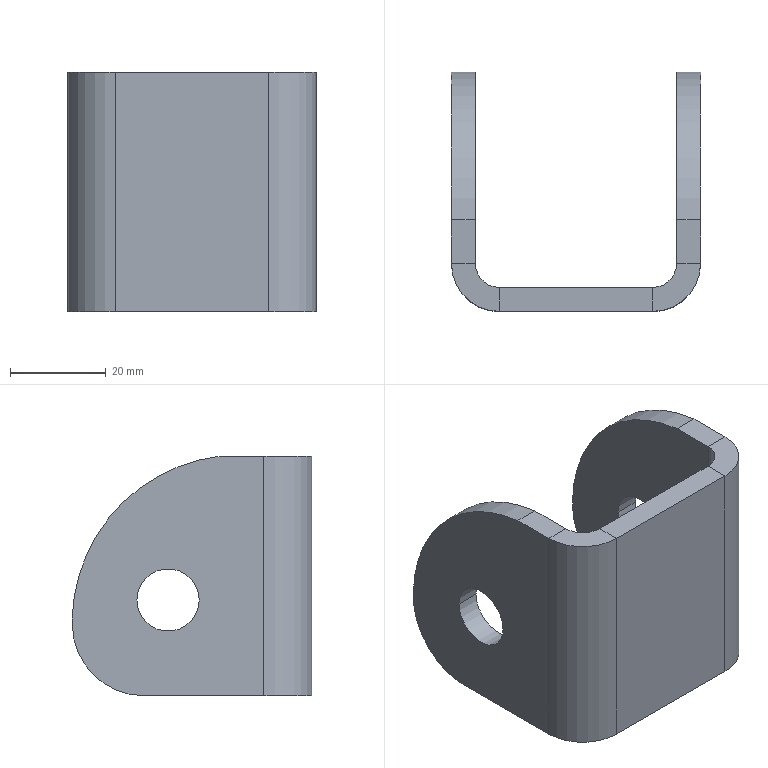Part | SolidWorks | features ICE 2, EdgeFlange 1, FlatPattern 1, SMBaseFlange 1, SheetMetal 1 | 1 solid | 30 faces | box 52 x 50 x 50 mm | volume 29535 mm3 | plane 18 | cylinder 12 | commonest cylinder face diameters 13 x4 10 x2 20 x2 30 x2 70 x2
STEP:
#1=CARTESIAN_POINT('',(26.,31.5,-5.));
#2=VERTEX_POINT('',#1);
#3=CARTESIAN_POINT('',(26.,18.5,-5.));
#4=VERTEX_POINT('',#3);
#5=CARTESIAN_POINT('',(26.,25.,-5.));
#6=DIRECTION('',(-1.,0.,0.));
#7=DIRECTION('',(0.,-1.,0.));
#8=AXIS2_PLACEMENT_3D('',#5,#6,#7);
#9=CIRCLE('',#8,6.5);
#10=EDGE_CURVE('',#2,#4,#9,.T.);
#11=ORIENTED_EDGE('',*,*,#10,.F.);
#12=CARTESIAN_POINT('',(21.,31.5,-5.));
#13=VERTEX_POINT('',#12);
#14=CARTESIAN_POINT('',(26.,31.5,-5.));
#15=DIRECTION('',(-1.,0.,0.));
#16=VECTOR('',#15,1000.);
#17=LINE('',#14,#16);
#18=EDGE_CURVE('',#2,#13,#17,.T.);
#19=ORIENTED_EDGE('',*,*,#18,.T.);
#20=CARTESIAN_POINT('',(21.,18.5,-5.));
#21=VERTEX_POINT('',#20);
#22=CARTESIAN_POINT('',(21.,25.,-5.));
#23=DIRECTION('',(1.,0.,0.));
#24=DIRECTION('',(0.,1.,0.));
#25=AXIS2_PLACEMENT_3D('',#22,#23,#24);
#26=CIRCLE('',#25,6.5);
#27=EDGE_CURVE('',#21,#13,#26,.T.);
#28=ORIENTED_EDGE('',*,*,#27,.F.);
#29=CARTESIAN_POINT('',(26.,18.5,-5.));
#30=DIRECTION('',(-1.,0.,0.));
#31=VECTOR('',#30,1000.);
#32=LINE('',#29,#31);
#33=EDGE_CURVE('',#4,#21,#32,.T.);
#34=ORIENTED_EDGE('',*,*,#33,.F.);
#35=EDGE_LOOP('',(#11,#19,#28,#34));
#36=FACE_OUTER_BOUND('',#35,.T.);
#37=CARTESIAN_POINT('',(26.,25.,-5.));
#38=DIRECTION('',(-1.,0.,0.));
#39=DIRECTION('',(0.,-1.,0.));
#40=AXIS2_PLACEMENT_3D('',#37,#38,#39);
#41=CYLINDRICAL_SURFACE('',#40,6.5);
#42=ADVANCED_FACE('',(#36),#41,.F.);
#43=CARTESIAN_POINT('',(-21.,18.5,-5.));
#44=VERTEX_POINT('',#43);
#45=CARTESIAN_POINT('',(-21.,31.5,-5.));
#46=VERTEX_POINT('',#45);
#47=CARTESIAN_POINT('',(-21.,25.,-5.));
#48=DIRECTION('',(1.,0.,0.));
#49=DIRECTION('',(0.,1.,0.));
#50=AXIS2_PLACEMENT_3D('',#47,#48,#49);
#51=CIRCLE('',#50,6.5);
#52=EDGE_CURVE('',#44,#46,#51,.T.);
#53=ORIENTED_EDGE('',*,*,#52,.T.);
#54=CARTESIAN_POINT('',(-26.,31.5,-5.));
#55=VERTEX_POINT('',#54);
#56=CARTESIAN_POINT('',(26.,31.5,-5.));
#57=DIRECTION('',(-1.,0.,0.));
#58=VECTOR('',#57,1000.);
#59=LINE('',#56,#58);
#60=EDGE_CURVE('',#46,#55,#59,.T.);
#61=ORIENTED_EDGE('',*,*,#60,.T.);
#62=CARTESIAN_POINT('',(-26.,18.5,-5.));
#63=VERTEX_POINT('',#62);
#64=CARTESIAN_POINT('',(-26.,25.,-5.));
#65=DIRECTION('',(-1.,0.,0.));
#66=DIRECTION('',(0.,-1.,0.));
#67=AXIS2_PLACEMENT_3D('',#64,#65,#66);
#68=CIRCLE('',#67,6.5);
#69=EDGE_CURVE('',#55,#63,#68,.T.);
#70=ORIENTED_EDGE('',*,*,#69,.T.);
#71=CARTESIAN_POINT('',(26.,18.5,-5.));
#72=DIRECTION('',(-1.,0.,0.));
#73=VECTOR('',#72,1000.);
#74=LINE('',#71,#73);
#75=EDGE_CURVE('',#44,#63,#74,.T.);
#76=ORIENTED_EDGE('',*,*,#75,.F.);
#77=EDGE_LOOP('',(#53,#61,#70,#76));
#78=FACE_OUTER_BOUND('',#77,.T.);
#79=CARTESIAN_POINT('',(26.,25.,-5.));
#80=DIRECTION('',(-1.,0.,0.));
#81=DIRECTION('',(0.,-1.,0.));
#82=AXIS2_PLACEMENT_3D('',#79,#80,#81);
#83=CYLINDRICAL_SURFACE('',#82,6.5);
#84=ADVANCED_FACE('',(#78),#83,.F.);
#85=CARTESIAN_POINT('',(21.,30.,-25.));
#86=VERTEX_POINT('',#85);
#87=CARTESIAN_POINT('',(21.,5.,-25.));
#88=VERTEX_POINT('',#87);
#89=CARTESIAN_POINT('',(21.,0.,-25.));
#90=DIRECTION('',(0.,-1.,0.));
#91=VECTOR('',#90,1000.);
#92=LINE('',#89,#91);
#93=EDGE_CURVE('',#86,#88,#92,.T.);
#94=ORIENTED_EDGE('',*,*,#93,.F.);
#95=CARTESIAN_POINT('',(26.,30.,-25.));
#96=VERTEX_POINT('',#95);
#97=CARTESIAN_POINT('',(26.,30.,-25.));
#98=DIRECTION('',(-1.,0.,0.));
#99=VECTOR('',#98,1000.);
#100=LINE('',#97,#99);
#101=EDGE_CURVE('',#96,#86,#100,.T.);
#102=ORIENTED_EDGE('',*,*,#101,.F.);
#103=CARTESIAN_POINT('',(26.,5.,-25.));
#104=VERTEX_POINT('',#103);
#105=CARTESIAN_POINT('',(26.,0.,-25.));
#106=DIRECTION('',(0.,-1.,0.));
#107=VECTOR('',#106,1000.);
#108=LINE('',#105,#107);
#109=EDGE_CURVE('',#96,#104,#108,.T.);
#110=ORIENTED_EDGE('',*,*,#109,.T.);
#111=CARTESIAN_POINT('',(21.,5.,-25.));
#112=DIRECTION('',(1.,0.,0.));
#113=VECTOR('',#112,1000.);
#114=LINE('',#111,#113);
#115=EDGE_CURVE('',#88,#104,#114,.T.);
#116=ORIENTED_EDGE('',*,*,#115,.F.);
#117=EDGE_LOOP('',(#94,#102,#110,#116));
#118=FACE_OUTER_BOUND('',#117,.T.);
#119=CARTESIAN_POINT('',(26.,0.,-25.));
#120=DIRECTION('',(0.,0.,-1.));
#121=DIRECTION('',(0.,1.,0.));
#122=AXIS2_PLACEMENT_3D('',#119,#120,#121);
#123=PLANE('',#122);
#124=ADVANCED_FACE('',(#118),#123,.T.);
#125=CARTESIAN_POINT('',(-26.,5.,-25.));
#126=VERTEX_POINT('',#125);
#127=CARTESIAN_POINT('',(-26.,30.,-25.));
#128=VERTEX_POINT('',#127);
#129=CARTESIAN_POINT('',(-26.,0.,-25.));
#130=DIRECTION('',(0.,1.,0.));
#131=VECTOR('',#130,1000.);
#132=LINE('',#129,#131);
#133=EDGE_CURVE('',#126,#128,#132,.T.);
#134=ORIENTED_EDGE('',*,*,#133,.T.);
#135=CARTESIAN_POINT('',(-21.,30.,-25.));
#136=VERTEX_POINT('',#135);
#137=CARTESIAN_POINT('',(26.,30.,-25.));
#138=DIRECTION('',(-1.,0.,0.));
#139=VECTOR('',#138,1000.);
#140=LINE('',#137,#139);
#141=EDGE_CURVE('',#136,#128,#140,.T.);
#142=ORIENTED_EDGE('',*,*,#141,.F.);
#143=CARTESIAN_POINT('',(-21.,5.,-25.));
#144=VERTEX_POINT('',#143);
#145=CARTESIAN_POINT('',(-21.,0.,-25.));
#146=DIRECTION('',(0.,1.,0.));
#147=VECTOR('',#146,1000.);
#148=LINE('',#145,#147);
#149=EDGE_CURVE('',#144,#136,#148,.T.);
#150=ORIENTED_EDGE('',*,*,#149,.F.);
#151=CARTESIAN_POINT('',(-26.,5.,-25.));
#152=DIRECTION('',(-1.,0.,0.));
#153=VECTOR('',#152,1000.);
#154=LINE('',#151,#153);
#155=EDGE_CURVE('',#144,#126,#154,.T.);
#156=ORIENTED_EDGE('',*,*,#155,.T.);
#157=EDGE_LOOP('',(#134,#142,#150,#156));
#158=FACE_OUTER_BOUND('',#157,.T.);
#159=CARTESIAN_POINT('',(-26.,0.,-25.));
#160=DIRECTION('',(0.,0.,-1.));
#161=DIRECTION('',(-1.,0.,0.));
#162=AXIS2_PLACEMENT_3D('',#159,#160,#161);
#163=PLANE('',#162);
#164=ADVANCED_FACE('',(#158),#163,.T.);
#165=CARTESIAN_POINT('',(-16.,-5.,25.));
#166=VERTEX_POINT('',#165);
#167=CARTESIAN_POINT('',(-16.,-5.,-25.));
#168=VERTEX_POINT('',#167);
#169=CARTESIAN_POINT('',(-16.,-5.,25.));
#170=DIRECTION('',(0.,0.,-1.));
#171=VECTOR('',#170,1000.);
#172=LINE('',#169,#171);
#173=EDGE_CURVE('',#166,#168,#172,.T.);
#174=ORIENTED_EDGE('',*,*,#173,.T.);
#175=CARTESIAN_POINT('',(16.,-5.,-25.));
#176=VERTEX_POINT('',#175);
#177=CARTESIAN_POINT('',(-26.,-5.,-25.));
#178=DIRECTION('',(-1.,0.,0.));
#179=VECTOR('',#178,1000.);
#180=LINE('',#177,#179);
#181=EDGE_CURVE('',#176,#168,#180,.T.);
#182=ORIENTED_EDGE('',*,*,#181,.F.);
#183=CARTESIAN_POINT('',(16.,-5.,25.));
#184=VERTEX_POINT('',#183);
#185=CARTESIAN_POINT('',(16.,-5.,-25.));
#186=DIRECTION('',(0.,0.,1.));
#187=VECTOR('',#186,1000.);
#188=LINE('',#185,#187);
#189=EDGE_CURVE('',#176,#184,#188,.T.);
#190=ORIENTED_EDGE('',*,*,#189,.T.);
#191=CARTESIAN_POINT('',(-26.,-5.,25.));
#192=DIRECTION('',(1.,0.,0.));
#193=VECTOR('',#192,1000.);
#194=LINE('',#191,#193);
#195=EDGE_CURVE('',#166,#184,#194,.T.);
#196=ORIENTED_EDGE('',*,*,#195,.F.);
#197=EDGE_LOOP('',(#174,#182,#190,#196));
#198=FACE_OUTER_BOUND('',#197,.T.);
#199=CARTESIAN_POINT('',(0.,-5.,0.));
#200=DIRECTION('',(0.,1.,0.));
#201=DIRECTION('',(0.,0.,1.));
#202=AXIS2_PLACEMENT_3D('',#199,#200,#201);
#203=PLANE('',#202);
#204=ADVANCED_FACE('',(#198),#203,.F.);
#205=CARTESIAN_POINT('',(16.,0.,-25.));
#206=VERTEX_POINT('',#205);
#207=CARTESIAN_POINT('',(-16.,0.,-25.));
#208=VERTEX_POINT('',#207);
#209=CARTESIAN_POINT('',(-26.,0.,-25.));
#210=DIRECTION('',(-1.,0.,0.));
#211=VECTOR('',#210,1000.);
#212=LINE('',#209,#211);
#213=EDGE_CURVE('',#206,#208,#212,.T.);
#214=ORIENTED_EDGE('',*,*,#213,.T.);
#215=CARTESIAN_POINT('',(-16.,0.,25.));
#216=VERTEX_POINT('',#215);
#217=CARTESIAN_POINT('',(-16.,0.,25.));
#218=DIRECTION('',(0.,0.,-1.));
#219=VECTOR('',#218,1000.);
#220=LINE('',#217,#219);
#221=EDGE_CURVE('',#216,#208,#220,.T.);
#222=ORIENTED_EDGE('',*,*,#221,.F.);
#223=CARTESIAN_POINT('',(16.,0.,25.));
#224=VERTEX_POINT('',#223);
#225=CARTESIAN_POINT('',(-26.,0.,25.));
#226=DIRECTION('',(1.,0.,0.));
#227=VECTOR('',#226,1000.);
#228=LINE('',#225,#227);
#229=EDGE_CURVE('',#216,#224,#228,.T.);
#230=ORIENTED_EDGE('',*,*,#229,.T.);
#231=CARTESIAN_POINT('',(16.,0.,-25.));
#232=DIRECTION('',(0.,0.,1.));
#233=VECTOR('',#232,1000.);
#234=LINE('',#231,#233);
#235=EDGE_CURVE('',#206,#224,#234,.T.);
#236=ORIENTED_EDGE('',*,*,#235,.F.);
#237=EDGE_LOOP('',(#214,#222,#230,#236));
#238=FACE_OUTER_BOUND('',#237,.T.);
#239=CARTESIAN_POINT('',(0.,0.,0.));
#240=DIRECTION('',(0.,1.,0.));
#241=DIRECTION('',(0.,0.,1.));
#242=AXIS2_PLACEMENT_3D('',#239,#240,#241);
#243=PLANE('',#242);
#244=ADVANCED_FACE('',(#238),#243,.T.);
#245=ORIENTED_EDGE('',*,*,#229,.F.);
#246=CARTESIAN_POINT('',(-16.,0.,25.));
#247=DIRECTION('',(0.,-1.,0.));
#248=VECTOR('',#247,1000.);
#249=LINE('',#246,#248);
#250=EDGE_CURVE('',#216,#166,#249,.T.);
#251=ORIENTED_EDGE('',*,*,#250,.T.);
#252=ORIENTED_EDGE('',*,*,#195,.T.);
#253=CARTESIAN_POINT('',(16.,0.,25.));
#254=DIRECTION('',(0.,-1.,0.));
#255=VECTOR('',#254,1000.);
#256=LINE('',#253,#255);
#257=EDGE_CURVE('',#224,#184,#256,.T.);
#258=ORIENTED_EDGE('',*,*,#257,.F.);
#259=EDGE_LOOP('',(#245,#251,#252,#258));
#260=FACE_OUTER_BOUND('',#259,.T.);
#261=CARTESIAN_POINT('',(-26.,-5.,25.));
#262=DIRECTION('',(0.,0.,1.));
#263=DIRECTION('',(1.,0.,0.));
#264=AXIS2_PLACEMENT_3D('',#261,#262,#263);
#265=PLANE('',#264);
#266=ADVANCED_FACE('',(#260),#265,.T.);
#267=CARTESIAN_POINT('',(-16.,0.,-25.));
#268=DIRECTION('',(0.,-1.,0.));
#269=VECTOR('',#268,1000.);
#270=LINE('',#267,#269);
#271=EDGE_CURVE('',#208,#168,#270,.T.);
#272=ORIENTED_EDGE('',*,*,#271,.F.);
#273=ORIENTED_EDGE('',*,*,#213,.F.);
#274=CARTESIAN_POINT('',(16.,0.,-25.));
#275=DIRECTION('',(0.,-1.,0.));
#276=VECTOR('',#275,1000.);
#277=LINE('',#274,#276);
#278=EDGE_CURVE('',#206,#176,#277,.T.);
#279=ORIENTED_EDGE('',*,*,#278,.T.);
#280=ORIENTED_EDGE('',*,*,#181,.T.);
#281=EDGE_LOOP('',(#272,#273,#279,#280));
#282=FACE_OUTER_BOUND('',#281,.T.);
#283=CARTESIAN_POINT('',(-26.,-5.,-25.));
#284=DIRECTION('',(0.,0.,-1.));
#285=DIRECTION('',(-1.,0.,0.));
#286=AXIS2_PLACEMENT_3D('',#283,#284,#285);
#287=PLANE('',#286);
#288=ADVANCED_FACE('',(#282),#287,.T.);
#289=CARTESIAN_POINT('',(21.,5.,25.));
#290=VERTEX_POINT('',#289);
#291=CARTESIAN_POINT('',(26.,5.,25.));
#292=VERTEX_POINT('',#291);
#293=CARTESIAN_POINT('',(26.,5.,25.));
#294=DIRECTION('',(1.,0.,0.));
#295=VECTOR('',#294,1000.);
#296=LINE('',#293,#295);
#297=EDGE_CURVE('',#290,#292,#296,.T.);
#298=ORIENTED_EDGE('',*,*,#297,.F.);
#299=CARTESIAN_POINT('',(16.,5.,25.));
#300=DIRECTION('',(0.,0.,1.));
#301=DIRECTION('',(-1.,0.,0.));
#302=AXIS2_PLACEMENT_3D('',#299,#300,#301);
#303=CIRCLE('',#302,5.);
#304=EDGE_CURVE('',#224,#290,#303,.T.);
#305=ORIENTED_EDGE('',*,*,#304,.F.);
#306=ORIENTED_EDGE('',*,*,#257,.T.);
#307=CARTESIAN_POINT('',(16.,5.,25.));
#308=DIRECTION('',(0.,0.,1.));
#309=DIRECTION('',(-1.,0.,0.));
#310=AXIS2_PLACEMENT_3D('',#307,#308,#309);
#311=CIRCLE('',#310,10.);
#312=EDGE_CURVE('',#184,#292,#311,.T.);
#313=ORIENTED_EDGE('',*,*,#312,.T.);
#314=EDGE_LOOP('',(#298,#305,#306,#313));
#315=FACE_OUTER_BOUND('',#314,.T.);
#316=CARTESIAN_POINT('',(16.,5.,25.));
#317=DIRECTION('',(0.,0.,1.));
#318=DIRECTION('',(1.,0.,0.));
#319=AXIS2_PLACEMENT_3D('',#316,#317,#318);
#320=PLANE('',#319);
#321=ADVANCED_FACE('',(#315),#320,.T.);
#322=CARTESIAN_POINT('',(16.,5.,-25.));
#323=DIRECTION('',(0.,0.,-1.));
#324=DIRECTION('',(-1.,0.,0.));
#325=AXIS2_PLACEMENT_3D('',#322,#323,#324);
#326=CIRCLE('',#325,5.);
#327=EDGE_CURVE('',#88,#206,#326,.T.);
#328=ORIENTED_EDGE('',*,*,#327,.F.);
#329=ORIENTED_EDGE('',*,*,#115,.T.);
#330=CARTESIAN_POINT('',(16.,5.,-25.));
#331=DIRECTION('',(0.,0.,-1.));
#332=DIRECTION('',(-1.,0.,0.));
#333=AXIS2_PLACEMENT_3D('',#330,#331,#332);
#334=CIRCLE('',#333,10.);
#335=EDGE_CURVE('',#104,#176,#334,.T.);
#336=ORIENTED_EDGE('',*,*,#335,.T.);
#337=ORIENTED_EDGE('',*,*,#278,.F.);
#338=EDGE_LOOP('',(#328,#329,#336,#337));
#339=FACE_OUTER_BOUND('',#338,.T.);
#340=CARTESIAN_POINT('',(16.,5.,-25.));
#341=DIRECTION('',(0.,0.,1.));
#342=DIRECTION('',(1.,0.,0.));
#343=AXIS2_PLACEMENT_3D('',#340,#341,#342);
#344=PLANE('',#343);
#345=ADVANCED_FACE('',(#339),#344,.F.);
#346=ORIENTED_EDGE('',*,*,#189,.F.);
#347=ORIENTED_EDGE('',*,*,#335,.F.);
#348=CARTESIAN_POINT('',(26.,5.,0.));
#349=DIRECTION('',(0.,0.,-1.));
#350=VECTOR('',#349,1000.);
#351=LINE('',#348,#350);
#352=EDGE_CURVE('',#292,#104,#351,.T.);
#353=ORIENTED_EDGE('',*,*,#352,.F.);
#354=ORIENTED_EDGE('',*,*,#312,.F.);
#355=EDGE_LOOP('',(#346,#347,#353,#354));
#356=FACE_OUTER_BOUND('',#355,.T.);
#357=CARTESIAN_POINT('',(16.,5.,-25.));
#358=DIRECTION('',(0.,0.,-1.));
#359=DIRECTION('',(1.,0.,0.));
#360=AXIS2_PLACEMENT_3D('',#357,#358,#359);
#361=CYLINDRICAL_SURFACE('',#360,10.);
#362=ADVANCED_FACE('',(#356),#361,.T.);
#363=ORIENTED_EDGE('',*,*,#235,.T.);
#364=ORIENTED_EDGE('',*,*,#304,.T.);
#365=CARTESIAN_POINT('',(21.,5.,25.));
#366=DIRECTION('',(0.,0.,-1.));
#367=VECTOR('',#366,1000.);
#368=LINE('',#365,#367);
#369=EDGE_CURVE('',#290,#88,#368,.T.);
#370=ORIENTED_EDGE('',*,*,#369,.T.);
#371=ORIENTED_EDGE('',*,*,#327,.T.);
#372=EDGE_LOOP('',(#363,#364,#370,#371));
#373=FACE_OUTER_BOUND('',#372,.T.);
#374=CARTESIAN_POINT('',(16.,5.,-25.));
#375=DIRECTION('',(0.,0.,-1.));
#376=DIRECTION('',(1.,0.,0.));
#377=AXIS2_PLACEMENT_3D('',#374,#375,#376);
#378=CYLINDRICAL_SURFACE('',#377,5.);
#379=ADVANCED_FACE('',(#373),#378,.F.);
#380=CARTESIAN_POINT('',(26.,14.151,25.));
#381=VERTEX_POINT('',#380);
#382=CARTESIAN_POINT('',(21.,14.151,25.));
#383=VERTEX_POINT('',#382);
#384=CARTESIAN_POINT('',(26.,14.151,25.));
#385=DIRECTION('',(-1.,0.,0.));
#386=VECTOR('',#385,1000.);
#387=LINE('',#384,#386);
#388=EDGE_CURVE('',#381,#383,#387,.T.);
#389=ORIENTED_EDGE('',*,*,#388,.T.);
#390=CARTESIAN_POINT('',(21.,0.,25.));
#391=DIRECTION('',(0.,1.,0.));
#392=VECTOR('',#391,1000.);
#393=LINE('',#390,#392);
#394=EDGE_CURVE('',#290,#383,#393,.T.);
#395=ORIENTED_EDGE('',*,*,#394,.F.);
#396=ORIENTED_EDGE('',*,*,#297,.T.);
#397=CARTESIAN_POINT('',(26.,45.,25.));
#398=DIRECTION('',(0.,1.,0.));
#399=VECTOR('',#398,1000.);
#400=LINE('',#397,#399);
#401=EDGE_CURVE('',#292,#381,#400,.T.);
#402=ORIENTED_EDGE('',*,*,#401,.T.);
#403=EDGE_LOOP('',(#389,#395,#396,#402));
#404=FACE_OUTER_BOUND('',#403,.T.);
#405=CARTESIAN_POINT('',(26.,45.,25.));
#406=DIRECTION('',(0.,0.,1.));
#407=DIRECTION('',(0.,-1.,0.));
#408=AXIS2_PLACEMENT_3D('',#405,#406,#407);
#409=PLANE('',#408);
#410=ADVANCED_FACE('',(#404),#409,.T.);
#411=CARTESIAN_POINT('',(26.,45.,-8.763));
#412=VERTEX_POINT('',#411);
#413=CARTESIAN_POINT('',(26.,10.014,-9.755));
#414=DIRECTION('',(1.,0.,0.));
#415=DIRECTION('',(0.,1.,0.));
#416=AXIS2_PLACEMENT_3D('',#413,#414,#415);
#417=CIRCLE('',#416,35.);
#418=EDGE_CURVE('',#412,#381,#417,.T.);
#419=ORIENTED_EDGE('',*,*,#418,.T.);
#420=ORIENTED_EDGE('',*,*,#401,.F.);
#421=ORIENTED_EDGE('',*,*,#352,.T.);
#422=ORIENTED_EDGE('',*,*,#109,.F.);
#423=CARTESIAN_POINT('',(26.,45.,-10.));
#424=VERTEX_POINT('',#423);
#425=CARTESIAN_POINT('',(26.,30.,-10.));
#426=DIRECTION('',(1.,0.,0.));
#427=DIRECTION('',(0.,1.,0.));
#428=AXIS2_PLACEMENT_3D('',#425,#426,#427);
#429=CIRCLE('',#428,15.);
#430=EDGE_CURVE('',#96,#424,#429,.T.);
#431=ORIENTED_EDGE('',*,*,#430,.T.);
#432=CARTESIAN_POINT('',(26.,45.,-25.));
#433=DIRECTION('',(0.,0.,-1.));
#434=VECTOR('',#433,1000.);
#435=LINE('',#432,#434);
#436=EDGE_CURVE('',#412,#424,#435,.T.);
#437=ORIENTED_EDGE('',*,*,#436,.F.);
#438=EDGE_LOOP('',(#419,#420,#421,#422,#431,#437));
#439=FACE_OUTER_BOUND('',#438,.T.);
#440=CARTESIAN_POINT('',(26.,25.,-5.));
#441=DIRECTION('',(-1.,0.,0.));
#442=DIRECTION('',(0.,-1.,0.));
#443=AXIS2_PLACEMENT_3D('',#440,#441,#442);
#444=CIRCLE('',#443,6.5);
#445=EDGE_CURVE('',#4,#2,#444,.T.);
#446=ORIENTED_EDGE('',*,*,#445,.T.);
#447=ORIENTED_EDGE('',*,*,#10,.T.);
#448=EDGE_LOOP('',(#446,#447));
#449=FACE_BOUND('',#448,.T.);
#450=CARTESIAN_POINT('',(26.,0.,0.));
#451=DIRECTION('',(1.,0.,0.));
#452=DIRECTION('',(0.,1.,0.));
#453=AXIS2_PLACEMENT_3D('',#450,#451,#452);
#454=PLANE('',#453);
#455=ADVANCED_FACE('',(#439,#449),#454,.T.);
#456=ORIENTED_EDGE('',*,*,#27,.T.);
#457=CARTESIAN_POINT('',(21.,25.,-5.));
#458=DIRECTION('',(1.,0.,0.));
#459=DIRECTION('',(0.,1.,0.));
#460=AXIS2_PLACEMENT_3D('',#457,#458,#459);
#461=CIRCLE('',#460,6.5);
#462=EDGE_CURVE('',#13,#21,#461,.T.);
#463=ORIENTED_EDGE('',*,*,#462,.T.);
#464=EDGE_LOOP('',(#456,#463));
#465=FACE_BOUND('',#464,.T.);
#466=ORIENTED_EDGE('',*,*,#394,.T.);
#467=CARTESIAN_POINT('',(21.,45.,-8.763));
#468=VERTEX_POINT('',#467);
#469=CARTESIAN_POINT('',(21.,10.014,-9.755));
#470=DIRECTION('',(-1.,0.,0.));
#471=DIRECTION('',(0.,1.,0.));
#472=AXIS2_PLACEMENT_3D('',#469,#470,#471);
#473=CIRCLE('',#472,35.);
#474=EDGE_CURVE('',#383,#468,#473,.T.);
#475=ORIENTED_EDGE('',*,*,#474,.T.);
#476=CARTESIAN_POINT('',(21.,45.,-10.));
#477=VERTEX_POINT('',#476);
#478=CARTESIAN_POINT('',(21.,45.,0.));
#479=DIRECTION('',(0.,0.,-1.));
#480=VECTOR('',#479,1000.);
#481=LINE('',#478,#480);
#482=EDGE_CURVE('',#468,#477,#481,.T.);
#483=ORIENTED_EDGE('',*,*,#482,.T.);
#484=CARTESIAN_POINT('',(21.,30.,-10.));
#485=DIRECTION('',(-1.,0.,0.));
#486=DIRECTION('',(0.,1.,0.));
#487=AXIS2_PLACEMENT_3D('',#484,#485,#486);
#488=CIRCLE('',#487,15.);
#489=EDGE_CURVE('',#477,#86,#488,.T.);
#490=ORIENTED_EDGE('',*,*,#489,.T.);
#491=ORIENTED_EDGE('',*,*,#93,.T.);
#492=ORIENTED_EDGE('',*,*,#369,.F.);
#493=EDGE_LOOP('',(#466,#475,#483,#490,#491,#492));
#494=FACE_OUTER_BOUND('',#493,.T.);
#495=CARTESIAN_POINT('',(21.,0.,0.));
#496=DIRECTION('',(1.,0.,0.));
#497=DIRECTION('',(0.,1.,0.));
#498=AXIS2_PLACEMENT_3D('',#495,#496,#497);
#499=PLANE('',#498);
#500=ADVANCED_FACE('',(#465,#494),#499,.F.);
#501=CARTESIAN_POINT('',(26.,45.,-8.763));
#502=DIRECTION('',(-1.,0.,0.));
#503=VECTOR('',#502,1000.);
#504=LINE('',#501,#503);
#505=EDGE_CURVE('',#412,#468,#504,.T.);
#506=ORIENTED_EDGE('',*,*,#505,.F.);
#507=ORIENTED_EDGE('',*,*,#436,.T.);
#508=CARTESIAN_POINT('',(26.,45.,-10.));
#509=DIRECTION('',(-1.,0.,0.));
#510=VECTOR('',#509,1000.);
#511=LINE('',#508,#510);
#512=EDGE_CURVE('',#424,#477,#511,.T.);
#513=ORIENTED_EDGE('',*,*,#512,.T.);
#514=ORIENTED_EDGE('',*,*,#482,.F.);
#515=EDGE_LOOP('',(#506,#507,#513,#514));
#516=FACE_OUTER_BOUND('',#515,.T.);
#517=CARTESIAN_POINT('',(26.,45.,-25.));
#518=DIRECTION('',(0.,1.,0.));
#519=DIRECTION('',(-1.,0.,0.));
#520=AXIS2_PLACEMENT_3D('',#517,#518,#519);
#521=PLANE('',#520);
#522=ADVANCED_FACE('',(#516),#521,.T.);
#523=ORIENTED_EDGE('',*,*,#155,.F.);
#524=CARTESIAN_POINT('',(-16.,5.,-25.));
#525=DIRECTION('',(0.,0.,-1.));
#526=DIRECTION('',(1.,0.,0.));
#527=AXIS2_PLACEMENT_3D('',#524,#525,#526);
#528=CIRCLE('',#527,5.);
#529=EDGE_CURVE('',#208,#144,#528,.T.);
#530=ORIENTED_EDGE('',*,*,#529,.F.);
#531=ORIENTED_EDGE('',*,*,#271,.T.);
#532=CARTESIAN_POINT('',(-16.,5.,-25.));
#533=DIRECTION('',(0.,0.,-1.));
#534=DIRECTION('',(1.,0.,0.));
#535=AXIS2_PLACEMENT_3D('',#532,#533,#534);
#536=CIRCLE('',#535,10.);
#537=EDGE_CURVE('',#168,#126,#536,.T.);
#538=ORIENTED_EDGE('',*,*,#537,.T.);
#539=EDGE_LOOP('',(#523,#530,#531,#538));
#540=FACE_OUTER_BOUND('',#539,.T.);
#541=CARTESIAN_POINT('',(-16.,5.,-25.));
#542=DIRECTION('',(0.,0.,-1.));
#543=DIRECTION('',(-1.,0.,0.));
#544=AXIS2_PLACEMENT_3D('',#541,#542,#543);
#545=PLANE('',#544);
#546=ADVANCED_FACE('',(#540),#545,.T.);
#547=CARTESIAN_POINT('',(-21.,5.,25.));
#548=VERTEX_POINT('',#547);
#549=CARTESIAN_POINT('',(-16.,5.,25.));
#550=DIRECTION('',(0.,0.,1.));
#551=DIRECTION('',(1.,0.,0.));
#552=AXIS2_PLACEMENT_3D('',#549,#550,#551);
#553=CIRCLE('',#552,5.);
#554=EDGE_CURVE('',#548,#216,#553,.T.);
#555=ORIENTED_EDGE('',*,*,#554,.F.);
#556=CARTESIAN_POINT('',(-26.,5.,25.));
#557=VERTEX_POINT('',#556);
#558=CARTESIAN_POINT('',(-21.,5.,25.));
#559=DIRECTION('',(-1.,0.,0.));
#560=VECTOR('',#559,1000.);
#561=LINE('',#558,#560);
#562=EDGE_CURVE('',#548,#557,#561,.T.);
#563=ORIENTED_EDGE('',*,*,#562,.T.);
#564=CARTESIAN_POINT('',(-16.,5.,25.));
#565=DIRECTION('',(0.,0.,1.));
#566=DIRECTION('',(1.,0.,0.));
#567=AXIS2_PLACEMENT_3D('',#564,#565,#566);
#568=CIRCLE('',#567,10.);
#569=EDGE_CURVE('',#557,#166,#568,.T.);
#570=ORIENTED_EDGE('',*,*,#569,.T.);
#571=ORIENTED_EDGE('',*,*,#250,.F.);
#572=EDGE_LOOP('',(#555,#563,#570,#571));
#573=FACE_OUTER_BOUND('',#572,.T.);
#574=CARTESIAN_POINT('',(-16.,5.,25.));
#575=DIRECTION('',(0.,0.,-1.));
#576=DIRECTION('',(-1.,0.,0.));
#577=AXIS2_PLACEMENT_3D('',#574,#575,#576);
#578=PLANE('',#577);
#579=ADVANCED_FACE('',(#573),#578,.F.);
#580=ORIENTED_EDGE('',*,*,#173,.F.);
#581=ORIENTED_EDGE('',*,*,#569,.F.);
#582=CARTESIAN_POINT('',(-26.,5.,-25.));
#583=DIRECTION('',(0.,0.,-1.));
#584=VECTOR('',#583,1000.);
#585=LINE('',#582,#584);
#586=EDGE_CURVE('',#557,#126,#585,.T.);
#587=ORIENTED_EDGE('',*,*,#586,.T.);
#588=ORIENTED_EDGE('',*,*,#537,.F.);
#589=EDGE_LOOP('',(#580,#581,#587,#588));
#590=FACE_OUTER_BOUND('',#589,.T.);
#591=CARTESIAN_POINT('',(-16.,5.,25.));
#592=DIRECTION('',(0.,0.,1.));
#593=DIRECTION('',(-1.,0.,0.));
#594=AXIS2_PLACEMENT_3D('',#591,#592,#593);
#595=CYLINDRICAL_SURFACE('',#594,10.);
#596=ADVANCED_FACE('',(#590),#595,.T.);
#597=ORIENTED_EDGE('',*,*,#221,.T.);
#598=ORIENTED_EDGE('',*,*,#529,.T.);
#599=CARTESIAN_POINT('',(-21.,5.,-25.));
#600=DIRECTION('',(0.,0.,1.));
#601=VECTOR('',#600,1000.);
#602=LINE('',#599,#601);
#603=EDGE_CURVE('',#144,#548,#602,.T.);
#604=ORIENTED_EDGE('',*,*,#603,.T.);
#605=ORIENTED_EDGE('',*,*,#554,.T.);
#606=EDGE_LOOP('',(#597,#598,#604,#605));
#607=FACE_OUTER_BOUND('',#606,.T.);
#608=CARTESIAN_POINT('',(-16.,5.,25.));
#609=DIRECTION('',(0.,0.,1.));
#610=DIRECTION('',(-1.,0.,0.));
#611=AXIS2_PLACEMENT_3D('',#608,#609,#610);
#612=CYLINDRICAL_SURFACE('',#611,5.);
#613=ADVANCED_FACE('',(#607),#612,.F.);
#614=CARTESIAN_POINT('',(-21.,14.151,25.));
#615=VERTEX_POINT('',#614);
#616=CARTESIAN_POINT('',(-26.,14.151,25.));
#617=VERTEX_POINT('',#616);
#618=CARTESIAN_POINT('',(26.,14.151,25.));
#619=DIRECTION('',(-1.,0.,0.));
#620=VECTOR('',#619,1000.);
#621=LINE('',#618,#620);
#622=EDGE_CURVE('',#615,#617,#621,.T.);
#623=ORIENTED_EDGE('',*,*,#622,.T.);
#624=CARTESIAN_POINT('',(-26.,45.,25.));
#625=DIRECTION('',(0.,-1.,0.));
#626=VECTOR('',#625,1000.);
#627=LINE('',#624,#626);
#628=EDGE_CURVE('',#617,#557,#627,.T.);
#629=ORIENTED_EDGE('',*,*,#628,.T.);
#630=ORIENTED_EDGE('',*,*,#562,.F.);
#631=CARTESIAN_POINT('',(-21.,0.,25.));
#632=DIRECTION('',(0.,-1.,0.));
#633=VECTOR('',#632,1000.);
#634=LINE('',#631,#633);
#635=EDGE_CURVE('',#615,#548,#634,.T.);
#636=ORIENTED_EDGE('',*,*,#635,.F.);
#637=EDGE_LOOP('',(#623,#629,#630,#636));
#638=FACE_OUTER_BOUND('',#637,.T.);
#639=CARTESIAN_POINT('',(-26.,45.,25.));
#640=DIRECTION('',(0.,0.,1.));
#641=DIRECTION('',(1.,0.,0.));
#642=AXIS2_PLACEMENT_3D('',#639,#640,#641);
#643=PLANE('',#642);
#644=ADVANCED_FACE('',(#638),#643,.T.);
#645=CARTESIAN_POINT('',(-26.,25.,-5.));
#646=DIRECTION('',(-1.,0.,0.));
#647=DIRECTION('',(0.,-1.,0.));
#648=AXIS2_PLACEMENT_3D('',#645,#646,#647);
#649=CIRCLE('',#648,6.5);
#650=EDGE_CURVE('',#63,#55,#649,.T.);
#651=ORIENTED_EDGE('',*,*,#650,.F.);
#652=ORIENTED_EDGE('',*,*,#69,.F.);
#653=EDGE_LOOP('',(#651,#652));
#654=FACE_BOUND('',#653,.T.);
#655=ORIENTED_EDGE('',*,*,#628,.F.);
#656=CARTESIAN_POINT('',(-26.,45.,-8.763));
#657=VERTEX_POINT('',#656);
#658=CARTESIAN_POINT('',(-26.,10.014,-9.755));
#659=DIRECTION('',(1.,0.,0.));
#660=DIRECTION('',(0.,1.,0.));
#661=AXIS2_PLACEMENT_3D('',#658,#659,#660);
#662=CIRCLE('',#661,35.);
#663=EDGE_CURVE('',#657,#617,#662,.T.);
#664=ORIENTED_EDGE('',*,*,#663,.F.);
#665=CARTESIAN_POINT('',(-26.,45.,-10.));
#666=VERTEX_POINT('',#665);
#667=CARTESIAN_POINT('',(-26.,45.,-25.));
#668=DIRECTION('',(0.,0.,1.));
#669=VECTOR('',#668,1000.);
#670=LINE('',#667,#669);
#671=EDGE_CURVE('',#666,#657,#670,.T.);
#672=ORIENTED_EDGE('',*,*,#671,.F.);
#673=CARTESIAN_POINT('',(-26.,30.,-10.));
#674=DIRECTION('',(1.,0.,0.));
#675=DIRECTION('',(0.,1.,0.));
#676=AXIS2_PLACEMENT_3D('',#673,#674,#675);
#677=CIRCLE('',#676,15.);
#678=EDGE_CURVE('',#128,#666,#677,.T.);
#679=ORIENTED_EDGE('',*,*,#678,.F.);
#680=ORIENTED_EDGE('',*,*,#133,.F.);
#681=ORIENTED_EDGE('',*,*,#586,.F.);
#682=EDGE_LOOP('',(#655,#664,#672,#679,#680,#681));
#683=FACE_OUTER_BOUND('',#682,.T.);
#684=CARTESIAN_POINT('',(-26.,0.,0.));
#685=DIRECTION('',(1.,0.,0.));
#686=DIRECTION('',(0.,1.,0.));
#687=AXIS2_PLACEMENT_3D('',#684,#685,#686);
#688=PLANE('',#687);
#689=ADVANCED_FACE('',(#654,#683),#688,.F.);
#690=CARTESIAN_POINT('',(-21.,45.,-8.763));
#691=VERTEX_POINT('',#690);
#692=CARTESIAN_POINT('',(-21.,10.014,-9.755));
#693=DIRECTION('',(-1.,0.,0.));
#694=DIRECTION('',(0.,1.,0.));
#695=AXIS2_PLACEMENT_3D('',#692,#693,#694);
#696=CIRCLE('',#695,35.);
#697=EDGE_CURVE('',#615,#691,#696,.T.);
#698=ORIENTED_EDGE('',*,*,#697,.F.);
#699=ORIENTED_EDGE('',*,*,#635,.T.);
#700=ORIENTED_EDGE('',*,*,#603,.F.);
#701=ORIENTED_EDGE('',*,*,#149,.T.);
#702=CARTESIAN_POINT('',(-21.,45.,-10.));
#703=VERTEX_POINT('',#702);
#704=CARTESIAN_POINT('',(-21.,30.,-10.));
#705=DIRECTION('',(-1.,0.,0.));
#706=DIRECTION('',(0.,1.,0.));
#707=AXIS2_PLACEMENT_3D('',#704,#705,#706);
#708=CIRCLE('',#707,15.);
#709=EDGE_CURVE('',#703,#136,#708,.T.);
#710=ORIENTED_EDGE('',*,*,#709,.F.);
#711=CARTESIAN_POINT('',(-21.,45.,0.));
#712=DIRECTION('',(0.,0.,1.));
#713=VECTOR('',#712,1000.);
#714=LINE('',#711,#713);
#715=EDGE_CURVE('',#703,#691,#714,.T.);
#716=ORIENTED_EDGE('',*,*,#715,.T.);
#717=EDGE_LOOP('',(#698,#699,#700,#701,#710,#716));
#718=FACE_OUTER_BOUND('',#717,.T.);
#719=ORIENTED_EDGE('',*,*,#52,.F.);
#720=CARTESIAN_POINT('',(-21.,25.,-5.));
#721=DIRECTION('',(1.,0.,0.));
#722=DIRECTION('',(0.,1.,0.));
#723=AXIS2_PLACEMENT_3D('',#720,#721,#722);
#724=CIRCLE('',#723,6.5);
#725=EDGE_CURVE('',#46,#44,#724,.T.);
#726=ORIENTED_EDGE('',*,*,#725,.F.);
#727=EDGE_LOOP('',(#719,#726));
#728=FACE_BOUND('',#727,.T.);
#729=CARTESIAN_POINT('',(-21.,0.,0.));
#730=DIRECTION('',(1.,0.,0.));
#731=DIRECTION('',(0.,1.,0.));
#732=AXIS2_PLACEMENT_3D('',#729,#730,#731);
#733=PLANE('',#732);
#734=ADVANCED_FACE('',(#718,#728),#733,.T.);
#735=CARTESIAN_POINT('',(26.,45.,-8.763));
#736=DIRECTION('',(-1.,0.,0.));
#737=VECTOR('',#736,1000.);
#738=LINE('',#735,#737);
#739=EDGE_CURVE('',#691,#657,#738,.T.);
#740=ORIENTED_EDGE('',*,*,#739,.F.);
#741=ORIENTED_EDGE('',*,*,#715,.F.);
#742=CARTESIAN_POINT('',(26.,45.,-10.));
#743=DIRECTION('',(1.,0.,0.));
#744=VECTOR('',#743,1000.);
#745=LINE('',#742,#744);
#746=EDGE_CURVE('',#666,#703,#745,.T.);
#747=ORIENTED_EDGE('',*,*,#746,.F.);
#748=ORIENTED_EDGE('',*,*,#671,.T.);
#749=EDGE_LOOP('',(#740,#741,#747,#748));
#750=FACE_OUTER_BOUND('',#749,.T.);
#751=CARTESIAN_POINT('',(-26.,45.,-25.));
#752=DIRECTION('',(0.,1.,0.));
#753=DIRECTION('',(-1.,0.,0.));
#754=AXIS2_PLACEMENT_3D('',#751,#752,#753);
#755=PLANE('',#754);
#756=ADVANCED_FACE('',(#750),#755,.T.);
#757=ORIENTED_EDGE('',*,*,#709,.T.);
#758=ORIENTED_EDGE('',*,*,#141,.T.);
#759=ORIENTED_EDGE('',*,*,#678,.T.);
#760=ORIENTED_EDGE('',*,*,#746,.T.);
#761=EDGE_LOOP('',(#757,#758,#759,#760));
#762=FACE_OUTER_BOUND('',#761,.T.);
#763=CARTESIAN_POINT('',(26.,30.,-10.));
#764=DIRECTION('',(-1.,0.,0.));
#765=DIRECTION('',(0.,-1.,0.));
#766=AXIS2_PLACEMENT_3D('',#763,#764,#765);
#767=CYLINDRICAL_SURFACE('',#766,15.);
#768=ADVANCED_FACE('',(#762),#767,.T.);
#769=ORIENTED_EDGE('',*,*,#60,.F.);
#770=ORIENTED_EDGE('',*,*,#725,.T.);
#771=ORIENTED_EDGE('',*,*,#75,.T.);
#772=ORIENTED_EDGE('',*,*,#650,.T.);
#773=EDGE_LOOP('',(#769,#770,#771,#772));
#774=FACE_OUTER_BOUND('',#773,.T.);
#775=CARTESIAN_POINT('',(26.,25.,-5.));
#776=DIRECTION('',(-1.,0.,0.));
#777=DIRECTION('',(0.,-1.,0.));
#778=AXIS2_PLACEMENT_3D('',#775,#776,#777);
#779=CYLINDRICAL_SURFACE('',#778,6.5);
#780=ADVANCED_FACE('',(#774),#779,.F.);
#781=ORIENTED_EDGE('',*,*,#512,.F.);
#782=ORIENTED_EDGE('',*,*,#430,.F.);
#783=ORIENTED_EDGE('',*,*,#101,.T.);
#784=ORIENTED_EDGE('',*,*,#489,.F.);
#785=EDGE_LOOP('',(#781,#782,#783,#784));
#786=FACE_OUTER_BOUND('',#785,.T.);
#787=CARTESIAN_POINT('',(26.,30.,-10.));
#788=DIRECTION('',(-1.,0.,0.));
#789=DIRECTION('',(0.,-1.,0.));
#790=AXIS2_PLACEMENT_3D('',#787,#788,#789);
#791=CYLINDRICAL_SURFACE('',#790,15.);
#792=ADVANCED_FACE('',(#786),#791,.T.);
#793=ORIENTED_EDGE('',*,*,#18,.F.);
#794=ORIENTED_EDGE('',*,*,#445,.F.);
#795=ORIENTED_EDGE('',*,*,#33,.T.);
#796=ORIENTED_EDGE('',*,*,#462,.F.);
#797=EDGE_LOOP('',(#793,#794,#795,#796));
#798=FACE_OUTER_BOUND('',#797,.T.);
#799=CARTESIAN_POINT('',(26.,25.,-5.));
#800=DIRECTION('',(-1.,0.,0.));
#801=DIRECTION('',(0.,-1.,0.));
#802=AXIS2_PLACEMENT_3D('',#799,#800,#801);
#803=CYLINDRICAL_SURFACE('',#802,6.5);
#804=ADVANCED_FACE('',(#798),#803,.F.);
#805=ORIENTED_EDGE('',*,*,#697,.T.);
#806=ORIENTED_EDGE('',*,*,#739,.T.);
#807=ORIENTED_EDGE('',*,*,#663,.T.);
#808=ORIENTED_EDGE('',*,*,#622,.F.);
#809=EDGE_LOOP('',(#805,#806,#807,#808));
#810=FACE_OUTER_BOUND('',#809,.T.);
#811=CARTESIAN_POINT('',(26.,10.014,-9.755));
#812=DIRECTION('',(-1.,0.,0.));
#813=DIRECTION('',(0.,-1.,0.));
#814=AXIS2_PLACEMENT_3D('',#811,#812,#813);
#815=CYLINDRICAL_SURFACE('',#814,35.);
#816=ADVANCED_FACE('',(#810),#815,.T.);
#817=ORIENTED_EDGE('',*,*,#388,.F.);
#818=ORIENTED_EDGE('',*,*,#418,.F.);
#819=ORIENTED_EDGE('',*,*,#505,.T.);
#820=ORIENTED_EDGE('',*,*,#474,.F.);
#821=EDGE_LOOP('',(#817,#818,#819,#820));
#822=FACE_OUTER_BOUND('',#821,.T.);
#823=CARTESIAN_POINT('',(26.,10.014,-9.755));
#824=DIRECTION('',(-1.,0.,0.));
#825=DIRECTION('',(0.,-1.,0.));
#826=AXIS2_PLACEMENT_3D('',#823,#824,#825);
#827=CYLINDRICAL_SURFACE('',#826,35.);
#828=ADVANCED_FACE('',(#822),#827,.T.);
#829=CLOSED_SHELL('',(#42,#84,#124,#164,#204,#244,#266,#288,#321,#345,#362,#379,#410,#455,#500,#522,#546,#579,#596,#613,#644,#689,#734,#756,#768,#780,#792,#804,#816,#828));
#830=MANIFOLD_SOLID_BREP('',#829);
#831=CARTESIAN_POINT('',(0.,0.,0.));
#832=DIRECTION('',(0.,0.,1.));
#833=DIRECTION('',(1.,0.,0.));
#834=AXIS2_PLACEMENT_3D('',#831,#832,#833);
#835=(LENGTH_UNIT()NAMED_UNIT(*)SI_UNIT(.MILLI.,.METRE.));
#836=UNCERTAINTY_MEASURE_WITH_UNIT(LENGTH_MEASURE(0.00001),#835,'','');
#837=(NAMED_UNIT(*)PLANE_ANGLE_UNIT()SI_UNIT($,.RADIAN.));
#838=(NAMED_UNIT(*)SI_UNIT($,.STERADIAN.)SOLID_ANGLE_UNIT());
#839=(GEOMETRIC_REPRESENTATION_CONTEXT(3)GLOBAL_UNCERTAINTY_ASSIGNED_CONTEXT((#836))GLOBAL_UNIT_ASSIGNED_CONTEXT((#835,#837,#838))REPRESENTATION_CONTEXT('',''));
#840=ADVANCED_BREP_SHAPE_REPRESENTATION('',(#830,#834),#839);